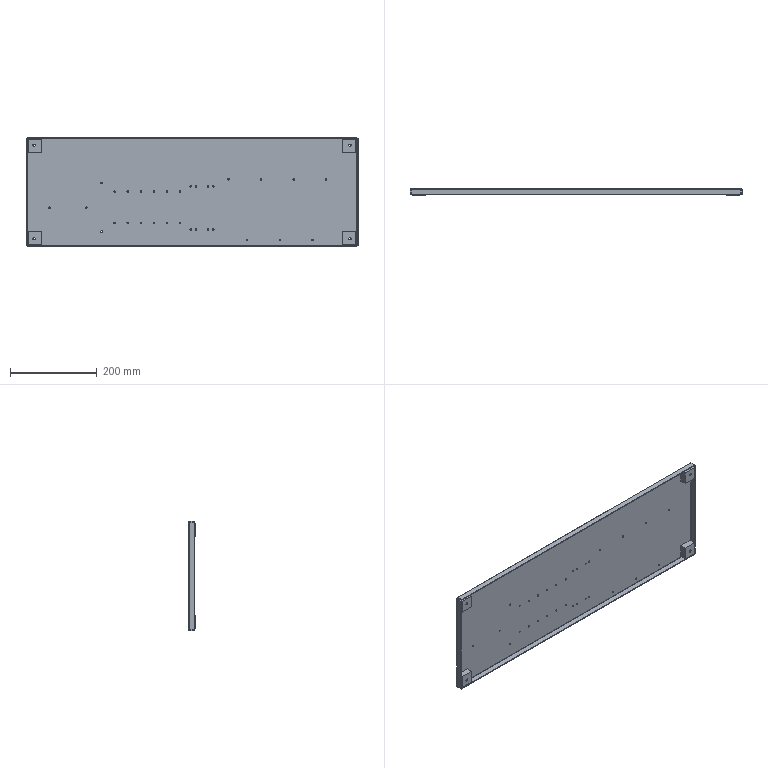Part | SolidWorks | features HoleWzd 6, LPattern 3, EdgeFlange 1, FlatPattern 1, ICE 1, SMBaseFlange 1, SheetMetal 1 | 1 solid | 144 faces | box 764 x 16 x 252 mm | volume 477309 mm3 | cylinder 88 | plane 46 | spline 8 | cone 2 | commonest cylinder face diameters 3.3 x60 5.5 x8 10 x8 1.473 x4 4 x4 5.473 x4